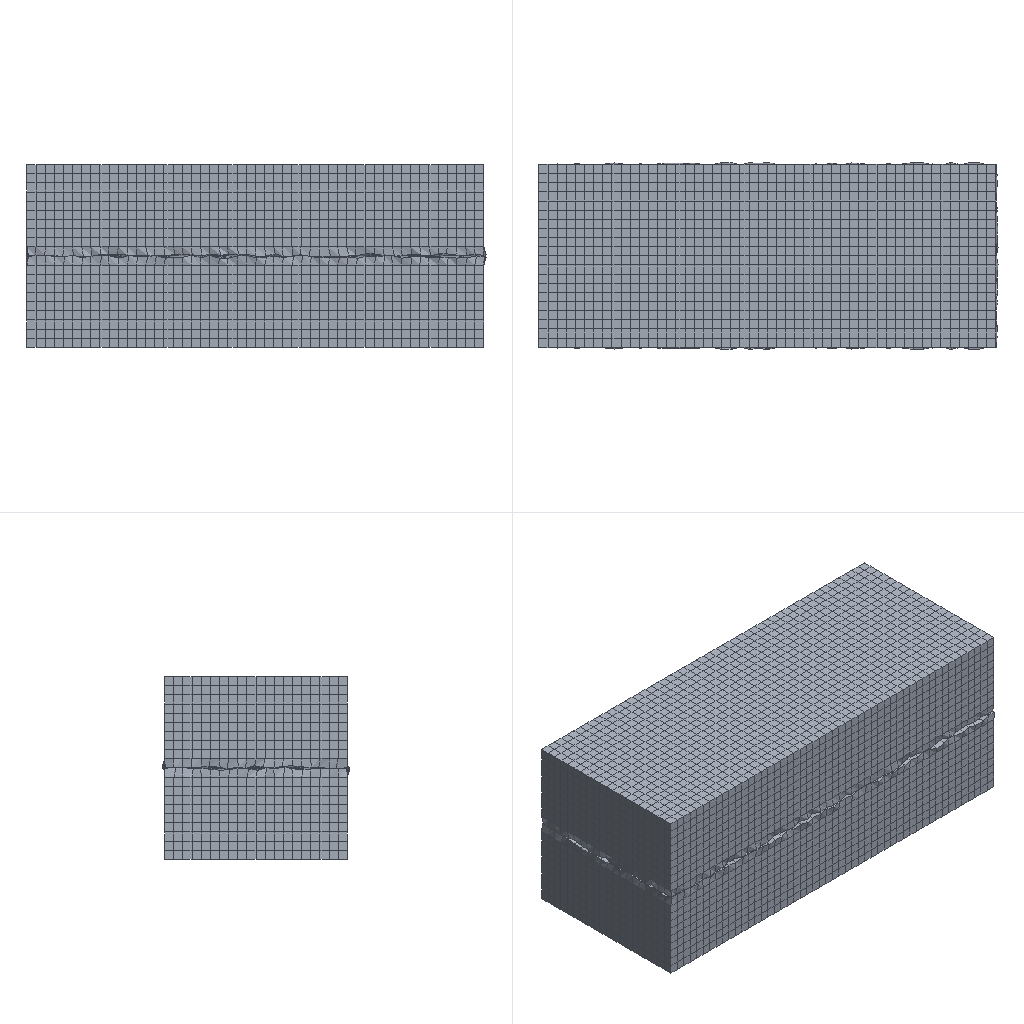Simulation study | abaqus
Set-up summary:
category,name,step,type,value,unit,region
solver,abaqus
solver,version,,,Abaqus/Standard 2020
units,not stated in the deck,,not stated
analysis,deck,,static,static
load_step,Step-1,Step-1,static
load_step,requested,,,1
mesh,nodes,,,23562
mesh,elements,,,20000
element_type,C3D8,,solid,20000
load,load commands in deck,,count,1
bc,support commands in deck,,count,5
material,MATERIAL-1,,in results
check,setup vs results,,match,"per instance, exact: element labels, types and connectivity; labels of the nodes the elements use; coordinates of those nodes at SINGLE_PRECISION in 1 of 2 instance(s)"
Abaqus input file, long lists of numbers shortened:
*Heading
** Job name: Job-2 Model name: Model-1-30mpa
** Generated by: Abaqus/CAE 2020
*Preprint, echo=NO, model=NO, history=NO, contact=NO
**
** PARTS
**
*Part, name=Part-1
*Node
      1,           0.,         -40.,          20.
      2,           0.,         -38.,          20.
** (11779 more lines like these left out)
*Element, type=C3D8
    1,   232,   233,   254,   253,     1,     2,    23,    22
    2,   233,   234,   255,   254,     2,     3,    24,    23
** (9998 more lines like these left out)
*Nset, nset=Set-2, generate
     1,  11781,      1
*Elset, elset=Set-2, generate
     1,  10000,      1
*Nset, nset=s2
   211,   212,   213,   214,   215,   216,   217,   218,   219,   220,   221,   222,   223,   224,   225,   226
   227,   228,   229,   230,   231,   442,   443,   444,   445,   446,   447,   448,   449,   450,   451,   452
** (65 more lines like these left out)
** Section: Section-1
*Solid Section, elset=Set-2, material=Material-1
,
*End Part
**
**
** ASSEMBLY
**
*Assembly, name=Assembly
**
*Instance, name=Part-1-1, part=Part-1
*End Instance
**
*Instance, name=Part-1-2, part=Part-1
          0.,         -40.,           0.
          0.,         -40.,           0.,           1.,         -40.,           0.,         180.
*End Instance
**
*Nset, nset=Set-1, instance=Part-1-1
     1,     2,     3,     4,     5,     6,     7,     8,     9,    10,    11,    12,    13,    14,    15,    16
    17,    18,    19,    20,    21,   232,   233,   234,   235,   236,   237,   238,   239,   240,   241,   242
** (65 more lines like these left out)
*Elset, elset=Set-1, instance=Part-1-1
    1,    2,    3,    4,    5,    6,    7,    8,    9,   10,   11,   12,   13,   14,   15,   16
   17,   18,   19,   20,  201,  202,  203,  204,  205,  206,  207,  208,  209,  210,  211,  212
** (61 more lines like these left out)
*Nset, nset=Set-2, instance=Part-1-1
     1,    21,    22,    42,    43,    63,    64,    84,    85,   105,   106,   126,   127,   147,   148,   168
   169,   189,   190,   210,   211,   231,   232,   252,   253,   273,   274,   294,   295,   315,   316,   336
** (69 more lines like these left out)
*Elset, elset=Set-2, instance=Part-1-1
     1,    20,    21,    40,    41,    60,    61,    80,    81,   100,   101,   120,   121,   140,   141,   160
   161,   180,   181,   200,   201,   220,   221,   240,   241,   260,   261,   280,   281,   300,   301,   320
** (61 more lines like these left out)
*Nset, nset=Set-3, instance=Part-1-1
     1,     2,     3,     4,     5,     6,     7,     8,     9,    10,    11,    12,    13,    14,    15,    16
    17,    18,    19,    20,    21,    22,    23,    24,    25,    26,    27,    28,    29,    30,    31,    32
** (27 more lines like these left out)
*Elset, elset=Set-3, instance=Part-1-1
     1,     2,     3,     4,     5,     6,     7,     8,     9,    10,    11,    12,    13,    14,    15,    16
    17,    18,    19,    20,    21,    22,    23,    24,    25,    26,    27,    28,    29,    30,    31,    32
** (23 more lines like these left out)
*Nset, nset=Set-4, instance=Part-1-2
     1,     2,     3,     4,     5,     6,     7,     8,     9,    10,    11,    12,    13,    14,    15,    16
    17,    18,    19,    20,    21,    22,    23,    24,    25,    26,    27,    28,    29,    30,    31,    32
** (27 more lines like these left out)
*Elset, elset=Set-4, instance=Part-1-2
     1,     2,     3,     4,     5,     6,     7,     8,     9,    10,    11,    12,    13,    14,    15,    16
    17,    18,    19,    20,    21,    22,    23,    24,    25,    26,    27,    28,    29,    30,    31,    32
** (23 more lines like these left out)
*Nset, nset=Set-5, instance=Part-1-2
     1,    21,    22,    42,    43,    63,    64,    84,    85,   105,   106,   126,   127,   147,   148,   168
   169,   189,   190,   210,   211,   231,   232,   252,   253,   273,   274,   294,   295,   315,   316,   336
** (69 more lines like these left out)
*Elset, elset=Set-5, instance=Part-1-2
     1,    20,    21,    40,    41,    60,    61,    80,    81,   100,   101,   120,   121,   140,   141,   160
   161,   180,   181,   200,   201,   220,   221,   240,   241,   260,   261,   280,   281,   300,   301,   320
** (61 more lines like these left out)
*Elset, elset=_Surf-1_S3, internal, instance=Part-1-2
    1,    2,    3,    4,    5,    6,    7,    8,    9,   10,   11,   12,   13,   14,   15,   16
   17,   18,   19,   20,  201,  202,  203,  204,  205,  206,  207,  208,  209,  210,  211,  212
** (61 more lines like these left out)
*Surface, type=ELEMENT, name=Surf-1
_Surf-1_S3, S3
*Elset, elset=_m_Surf-2_S5, internal, instance=Part-1-1
   181,   182,   183,   184,   185,   186,   187,   188,   189,   190,   191,   192,   193,   194,   195,   196
   197,   198,   199,   200,   381,   382,   383,   384,   385,   386,   387,   388,   389,   390,   391,   392
** (61 more lines like these left out)
*Surface, type=ELEMENT, name=m_Surf-2
_m_Surf-2_S5, S5
*Elset, elset=_s_Surf-2_S5, internal, instance=Part-1-2
   181,   182,   183,   184,   185,   186,   187,   188,   189,   190,   191,   192,   193,   194,   195,   196
   197,   198,   199,   200,   381,   382,   383,   384,   385,   386,   387,   388,   389,   390,   391,   392
** (61 more lines like these left out)
*Surface, type=ELEMENT, name=s_Surf-2
_s_Surf-2_S5, S5
*End Assembly
*Amplitude, name=Amp-1
             0.,              0.,              1.,              1.
**
** MATERIALS
**
*Material, name=Material-1
*Elastic
20000., 0.25
*Plastic
300.,0.
**
** INTERACTION PROPERTIES
**
*Surface Interaction, name=IntProp-1
1.,
*Friction, slip tolerance=0.005
 0.4,
*Surface Behavior, pressure-overclosure=HARD
**
** INTERACTIONS
**
** Interaction: Int-1
*Contact Pair, interaction=IntProp-1, type=SURFACE TO SURFACE
s_Surf-2, m_Surf-2
** ----------------------------------------------------------------
**
** STEP: Step-1
**
*Step, name=Step-1, nlgeom=YES, inc=1000
*Static, stabilize=0.0002, allsdtol=0.05, continue=NO
0.01, 1., 1e-05, 1.
**
** BOUNDARY CONDITIONS
**
** Name: BC-1 Type: 位移/转角
*Boundary
Set-1, 3, 3
** Name: BC-2 Type: 对称/反对称/完全固定
*Boundary
Set-2, YSYMM
** Name: BC-3 Type: 对称/反对称/完全固定
*Boundary
Set-3, XSYMM
** Name: BC-4 Type: 对称/反对称/完全固定
*Boundary
Set-4, XSYMM
** Name: BC-5 Type: 对称/反对称/完全固定
*Boundary
Set-5, YSYMM
**
** LOADS
**
** Name: Load-1   Type: Pressure
*Dsload, amplitude=Amp-1
Surf-1, P, 30.
**
** OUTPUT REQUESTS
**
*Restart, write, frequency=0
**
** FIELD OUTPUT: F-Output-1
**
*Output, field
*Node Output
CF, RF, U, V
*Element Output, directions=YES
E, LE, MISES, PE, PEEQ, PEMAG, S
*Contact Output
CDISP, CSTRESS
**
** HISTORY OUTPUT: H-Output-1
**
*Output, history, variable=PRESELECT
*End Step
Results summary:
result,step,,completed,increments=11 time=1.0/1.0
result,analysis,,,static
result,last_loadstep,,,1
result,primary field,,,U
result,reaction total,,FX,33.14,model units
result,reaction total,,FY,3.845,model units
result,reaction total,,FZ,-119683.75,model units